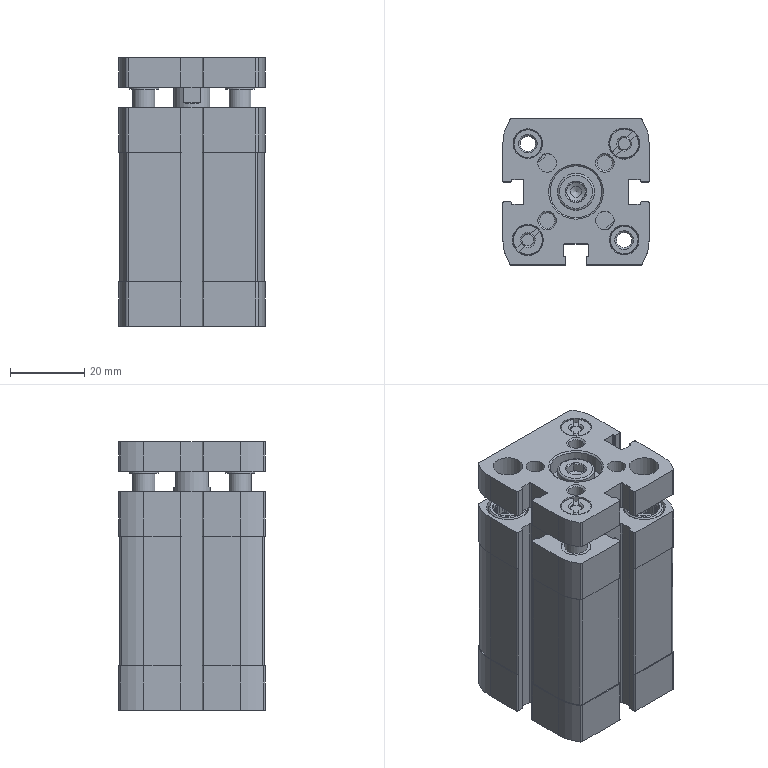Part | NX | features BREP 2 | 2 solids | 501 faces | box 39.5 x 39.5 x 72.5 mm | volume 80478 mm3 | plane 301 | cylinder 154 | cone 43 | torus 3 | commonest cylinder face diameters 0.8 x36 0.4 x24 1.6 x16 23.4 x16 4.134 x10 8 x8